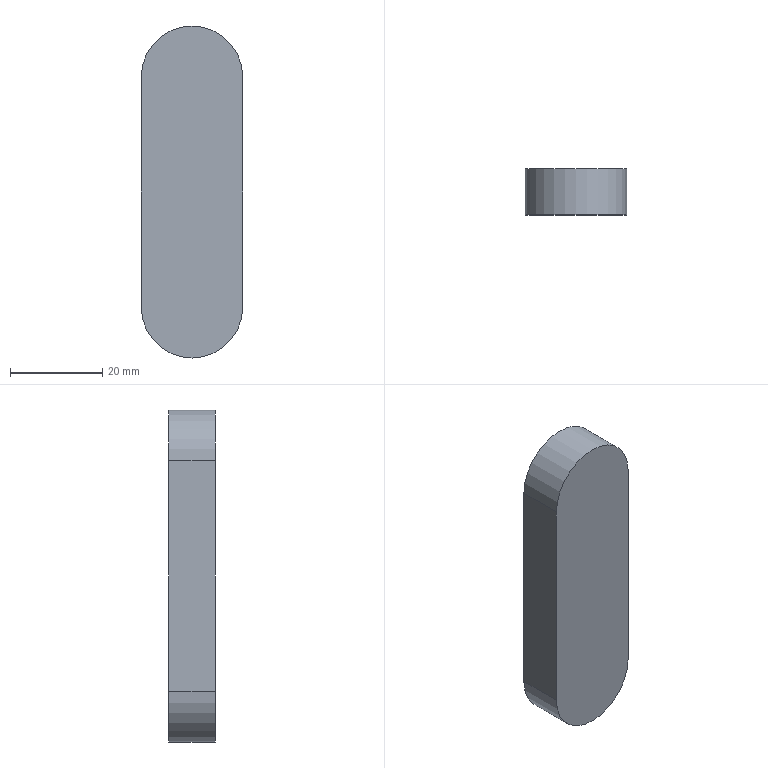Part | SolidWorks | features Extrusion 1 | 1 solid | 7 faces | box 22 x 10 x 72 mm | volume 14801 mm3 | plane 4 | cylinder 3 | commonest cylinder face diameters 22 x3
STEP:
#1=CARTESIAN_POINT('',(0.,10.,-36.));
#2=VERTEX_POINT('',#1);
#3=CARTESIAN_POINT('',(-11.,10.,-25.));
#4=VERTEX_POINT('',#3);
#5=CARTESIAN_POINT('',(0.,10.,-25.));
#6=DIRECTION('',(0.,1.,0.));
#7=DIRECTION('',(0.,0.,1.));
#8=AXIS2_PLACEMENT_3D('',#5,#6,#7);
#9=CIRCLE('',#8,11.);
#10=EDGE_CURVE('',#2,#4,#9,.T.);
#11=ORIENTED_EDGE('',*,*,#10,.F.);
#12=CARTESIAN_POINT('',(0.,0.,-36.));
#13=VERTEX_POINT('',#12);
#14=CARTESIAN_POINT('',(0.,10.,-36.));
#15=DIRECTION('',(0.,-1.,0.));
#16=VECTOR('',#15,1000.);
#17=LINE('',#14,#16);
#18=EDGE_CURVE('',#2,#13,#17,.T.);
#19=ORIENTED_EDGE('',*,*,#18,.T.);
#20=CARTESIAN_POINT('',(-11.,0.,-25.));
#21=VERTEX_POINT('',#20);
#22=CARTESIAN_POINT('',(0.,0.,-25.));
#23=DIRECTION('',(0.,1.,0.));
#24=DIRECTION('',(0.,0.,1.));
#25=AXIS2_PLACEMENT_3D('',#22,#23,#24);
#26=CIRCLE('',#25,11.);
#27=EDGE_CURVE('',#13,#21,#26,.T.);
#28=ORIENTED_EDGE('',*,*,#27,.T.);
#29=CARTESIAN_POINT('',(-11.,10.,-25.));
#30=DIRECTION('',(0.,-1.,0.));
#31=VECTOR('',#30,1000.);
#32=LINE('',#29,#31);
#33=EDGE_CURVE('',#4,#21,#32,.T.);
#34=ORIENTED_EDGE('',*,*,#33,.F.);
#35=EDGE_LOOP('',(#11,#19,#28,#34));
#36=FACE_OUTER_BOUND('',#35,.T.);
#37=CARTESIAN_POINT('',(0.,10.,-25.));
#38=DIRECTION('',(0.,-1.,0.));
#39=DIRECTION('',(0.,0.,-1.));
#40=AXIS2_PLACEMENT_3D('',#37,#38,#39);
#41=CYLINDRICAL_SURFACE('',#40,11.);
#42=ADVANCED_FACE('',(#36),#41,.T.);
#43=CARTESIAN_POINT('',(-11.,0.,25.));
#44=VERTEX_POINT('',#43);
#45=CARTESIAN_POINT('',(11.,0.,25.));
#46=VERTEX_POINT('',#45);
#47=CARTESIAN_POINT('',(0.,0.,25.));
#48=DIRECTION('',(0.,1.,0.));
#49=DIRECTION('',(0.,0.,1.));
#50=AXIS2_PLACEMENT_3D('',#47,#48,#49);
#51=CIRCLE('',#50,11.);
#52=EDGE_CURVE('',#44,#46,#51,.T.);
#53=ORIENTED_EDGE('',*,*,#52,.T.);
#54=CARTESIAN_POINT('',(11.,10.,25.));
#55=VERTEX_POINT('',#54);
#56=CARTESIAN_POINT('',(11.,10.,25.));
#57=DIRECTION('',(0.,-1.,0.));
#58=VECTOR('',#57,1000.);
#59=LINE('',#56,#58);
#60=EDGE_CURVE('',#55,#46,#59,.T.);
#61=ORIENTED_EDGE('',*,*,#60,.F.);
#62=CARTESIAN_POINT('',(-11.,10.,25.));
#63=VERTEX_POINT('',#62);
#64=CARTESIAN_POINT('',(0.,10.,25.));
#65=DIRECTION('',(0.,1.,0.));
#66=DIRECTION('',(0.,0.,1.));
#67=AXIS2_PLACEMENT_3D('',#64,#65,#66);
#68=CIRCLE('',#67,11.);
#69=EDGE_CURVE('',#63,#55,#68,.T.);
#70=ORIENTED_EDGE('',*,*,#69,.F.);
#71=CARTESIAN_POINT('',(-11.,10.,25.));
#72=DIRECTION('',(0.,-1.,0.));
#73=VECTOR('',#72,1000.);
#74=LINE('',#71,#73);
#75=EDGE_CURVE('',#63,#44,#74,.T.);
#76=ORIENTED_EDGE('',*,*,#75,.T.);
#77=EDGE_LOOP('',(#53,#61,#70,#76));
#78=FACE_OUTER_BOUND('',#77,.T.);
#79=CARTESIAN_POINT('',(0.,10.,25.));
#80=DIRECTION('',(0.,-1.,0.));
#81=DIRECTION('',(0.,0.,-1.));
#82=AXIS2_PLACEMENT_3D('',#79,#80,#81);
#83=CYLINDRICAL_SURFACE('',#82,11.);
#84=ADVANCED_FACE('',(#78),#83,.T.);
#85=CARTESIAN_POINT('',(11.,0.,-25.));
#86=VERTEX_POINT('',#85);
#87=CARTESIAN_POINT('',(11.,0.,25.));
#88=DIRECTION('',(0.,0.,-1.));
#89=VECTOR('',#88,1000.);
#90=LINE('',#87,#89);
#91=EDGE_CURVE('',#46,#86,#90,.T.);
#92=ORIENTED_EDGE('',*,*,#91,.T.);
#93=CARTESIAN_POINT('',(11.,10.,-25.));
#94=VERTEX_POINT('',#93);
#95=CARTESIAN_POINT('',(11.,10.,-25.));
#96=DIRECTION('',(0.,-1.,0.));
#97=VECTOR('',#96,1000.);
#98=LINE('',#95,#97);
#99=EDGE_CURVE('',#94,#86,#98,.T.);
#100=ORIENTED_EDGE('',*,*,#99,.F.);
#101=CARTESIAN_POINT('',(11.,10.,25.));
#102=DIRECTION('',(0.,0.,-1.));
#103=VECTOR('',#102,1000.);
#104=LINE('',#101,#103);
#105=EDGE_CURVE('',#55,#94,#104,.T.);
#106=ORIENTED_EDGE('',*,*,#105,.F.);
#107=ORIENTED_EDGE('',*,*,#60,.T.);
#108=EDGE_LOOP('',(#92,#100,#106,#107));
#109=FACE_OUTER_BOUND('',#108,.T.);
#110=CARTESIAN_POINT('',(11.,10.,25.));
#111=DIRECTION('',(-1.,0.,0.));
#112=DIRECTION('',(0.,0.,1.));
#113=AXIS2_PLACEMENT_3D('',#110,#111,#112);
#114=PLANE('',#113);
#115=ADVANCED_FACE('',(#109),#114,.F.);
#116=ORIENTED_EDGE('',*,*,#18,.F.);
#117=CARTESIAN_POINT('',(0.,10.,-25.));
#118=DIRECTION('',(0.,1.,0.));
#119=DIRECTION('',(0.,0.,1.));
#120=AXIS2_PLACEMENT_3D('',#117,#118,#119);
#121=CIRCLE('',#120,11.);
#122=EDGE_CURVE('',#94,#2,#121,.T.);
#123=ORIENTED_EDGE('',*,*,#122,.F.);
#124=ORIENTED_EDGE('',*,*,#99,.T.);
#125=CARTESIAN_POINT('',(0.,0.,-25.));
#126=DIRECTION('',(0.,1.,0.));
#127=DIRECTION('',(0.,0.,1.));
#128=AXIS2_PLACEMENT_3D('',#125,#126,#127);
#129=CIRCLE('',#128,11.);
#130=EDGE_CURVE('',#86,#13,#129,.T.);
#131=ORIENTED_EDGE('',*,*,#130,.T.);
#132=EDGE_LOOP('',(#116,#123,#124,#131));
#133=FACE_OUTER_BOUND('',#132,.T.);
#134=CARTESIAN_POINT('',(0.,10.,-25.));
#135=DIRECTION('',(0.,-1.,0.));
#136=DIRECTION('',(0.,0.,-1.));
#137=AXIS2_PLACEMENT_3D('',#134,#135,#136);
#138=CYLINDRICAL_SURFACE('',#137,11.);
#139=ADVANCED_FACE('',(#133),#138,.T.);
#140=CARTESIAN_POINT('',(-11.,0.,25.));
#141=DIRECTION('',(0.,0.,1.));
#142=VECTOR('',#141,1000.);
#143=LINE('',#140,#142);
#144=EDGE_CURVE('',#21,#44,#143,.T.);
#145=ORIENTED_EDGE('',*,*,#144,.T.);
#146=ORIENTED_EDGE('',*,*,#75,.F.);
#147=CARTESIAN_POINT('',(-11.,10.,25.));
#148=DIRECTION('',(0.,0.,1.));
#149=VECTOR('',#148,1000.);
#150=LINE('',#147,#149);
#151=EDGE_CURVE('',#4,#63,#150,.T.);
#152=ORIENTED_EDGE('',*,*,#151,.F.);
#153=ORIENTED_EDGE('',*,*,#33,.T.);
#154=EDGE_LOOP('',(#145,#146,#152,#153));
#155=FACE_OUTER_BOUND('',#154,.T.);
#156=CARTESIAN_POINT('',(-11.,10.,25.));
#157=DIRECTION('',(1.,0.,0.));
#158=DIRECTION('',(0.,0.,-1.));
#159=AXIS2_PLACEMENT_3D('',#156,#157,#158);
#160=PLANE('',#159);
#161=ADVANCED_FACE('',(#155),#160,.F.);
#162=ORIENTED_EDGE('',*,*,#69,.T.);
#163=ORIENTED_EDGE('',*,*,#105,.T.);
#164=ORIENTED_EDGE('',*,*,#122,.T.);
#165=ORIENTED_EDGE('',*,*,#10,.T.);
#166=ORIENTED_EDGE('',*,*,#151,.T.);
#167=EDGE_LOOP('',(#162,#163,#164,#165,#166));
#168=FACE_OUTER_BOUND('',#167,.T.);
#169=CARTESIAN_POINT('',(0.,10.,25.));
#170=DIRECTION('',(0.,1.,0.));
#171=DIRECTION('',(0.,0.,1.));
#172=AXIS2_PLACEMENT_3D('',#169,#170,#171);
#173=PLANE('',#172);
#174=ADVANCED_FACE('',(#168),#173,.T.);
#175=ORIENTED_EDGE('',*,*,#52,.F.);
#176=ORIENTED_EDGE('',*,*,#144,.F.);
#177=ORIENTED_EDGE('',*,*,#27,.F.);
#178=ORIENTED_EDGE('',*,*,#130,.F.);
#179=ORIENTED_EDGE('',*,*,#91,.F.);
#180=EDGE_LOOP('',(#175,#176,#177,#178,#179));
#181=FACE_OUTER_BOUND('',#180,.T.);
#182=CARTESIAN_POINT('',(0.,0.,25.));
#183=DIRECTION('',(0.,1.,0.));
#184=DIRECTION('',(0.,0.,1.));
#185=AXIS2_PLACEMENT_3D('',#182,#183,#184);
#186=PLANE('',#185);
#187=ADVANCED_FACE('',(#181),#186,.F.);
#188=CLOSED_SHELL('',(#42,#84,#115,#139,#161,#174,#187));
#189=MANIFOLD_SOLID_BREP('',#188);
#190=CARTESIAN_POINT('',(0.,0.,0.));
#191=DIRECTION('',(0.,0.,1.));
#192=DIRECTION('',(1.,0.,0.));
#193=AXIS2_PLACEMENT_3D('',#190,#191,#192);
#194=(LENGTH_UNIT()NAMED_UNIT(*)SI_UNIT(.MILLI.,.METRE.));
#195=UNCERTAINTY_MEASURE_WITH_UNIT(LENGTH_MEASURE(0.00001),#194,'','');
#196=(NAMED_UNIT(*)PLANE_ANGLE_UNIT()SI_UNIT($,.RADIAN.));
#197=(NAMED_UNIT(*)SI_UNIT($,.STERADIAN.)SOLID_ANGLE_UNIT());
#198=(GEOMETRIC_REPRESENTATION_CONTEXT(3)GLOBAL_UNCERTAINTY_ASSIGNED_CONTEXT((#195))GLOBAL_UNIT_ASSIGNED_CONTEXT((#194,#196,#197))REPRESENTATION_CONTEXT('',''));
#199=ADVANCED_BREP_SHAPE_REPRESENTATION('',(#189,#193),#198);